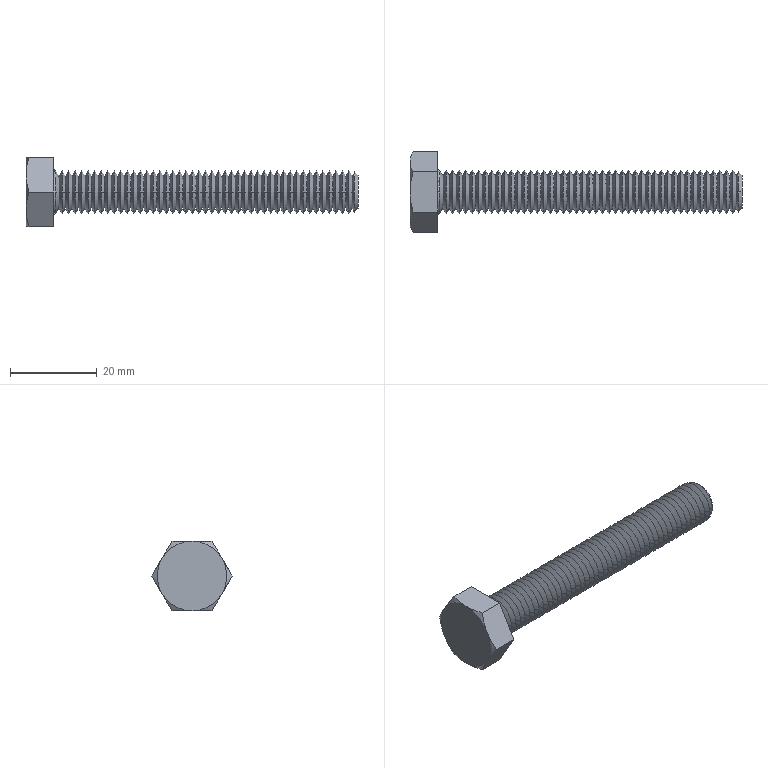Part | STEP file | GB/T 5783 M10×70 | 1 solid | 293 faces | box 76.4 x 18.475 x 16 mm | volume 5610 mm3 | cone 192 | cylinder 90 | plane 9 | torus 2 | commonest cylinder face diameters 10 x90